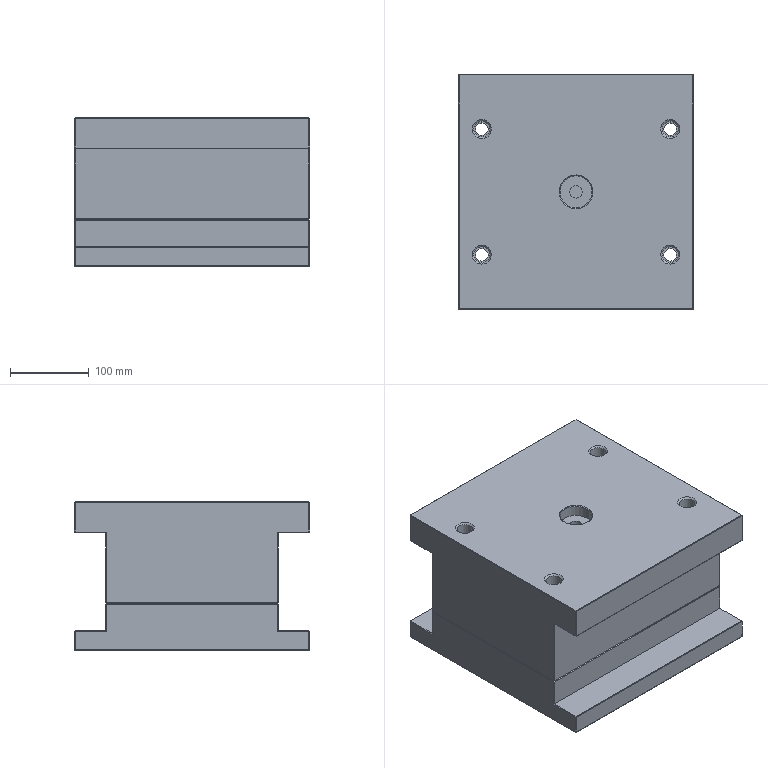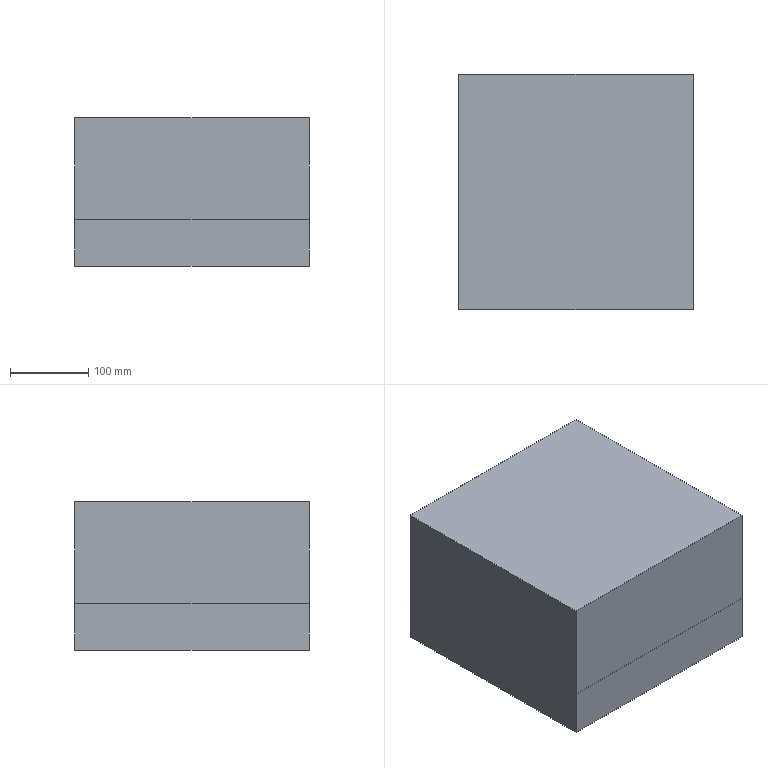CAM job | NX | 3-axis milling, drilling | part box 300 x 300 x 190 mm | stock box 300 x 300 x 190 mm
Tools:
number,name,description,diameter,corner_radius,flute_length,length,flutes
7,D6A45,Milling Tool-5 Parameters,6.0,0.0,50.0,75.0,2
1,ZXZ,Milling Tool-5 Parameters,6.0,0.0,50.0,75.0,2
11,10.ZT,Drilling Tool,10.0,0.0,35.0,50.0,2
2,D25R5,Milling Tool-5 Parameters,25.0,5.0,50.0,75.0,2
10,D10C,Milling Tool-5 Parameters,10.0,0.0,50.0,75.0,2
9,D10JING,Milling Tool-5 Parameters,10.0,0.0,50.0,75.0,2
12,R3,Milling Tool-5 Parameters,6.0,3.0,50.0,75.0,2
6,D6,Milling Tool-5 Parameters,6.0,0.0,50.0,75.0,2
15,D25R0.8,Milling Tool-5 Parameters,25.0,0.8,50.0,75.0,2
Operations:
program,operation,operation_type,tool,method,geometry_group,spindle_rpm,surface_speed,feed_per_tooth,feed_cut,feed_plunge,cut_length_mm,path_length_mm,cut_time_min,machine_time_min
1,DRILLING,Operation,ZXZ,METHOD,A,3500.0,65.0,0.0286,200.0,0.0,20.0,720.563,0.1,0.1701
1,DRILLING_1,Operation,10.ZT,METHOD,A,1200.0,37.0,0.05,120.0,0.0,268.017,1165.109,2.233,2.323
1,CAVITY_MILL,CavityMilling,D25R5,METHOD,A,1000.0,78.0,1.0,2000.0,1000.0,41589.871,44517.635,22.589,22.882
1,FLOOR_WALL,VolumeBased25DMillingOperation,D25R5,METHOD,A,1000.0,0.0,0.0,2000.0,1000.0,248046.214,253706.579,125.799,126.365
1,CAVITY_MILL_COPY,CavityMilling,D10C,METHOD,A,2500.0,78.0,0.4,2000.0,1000.0,24468.781,47953.241,12.498,14.847
1,HOLE_MILLING,CylinderMilling,D10C,METHOD,A,2000.0,62.0,0.375,1500.0,100.0,22158.353,23196.353,14.772,14.876
1,FLOOR_WALL_1,VolumeBased25DMillingOperation,D10JING,METHOD,A,4000.0,125.0,0.15,1200.0,100.0,5645.915,6426.663,4.705,4.783
1,FLOOR_WALL_1_COPY,VolumeBased25DMillingOperation,D10JING,METHOD,A,4000.0,125.0,0.15,1200.0,100.0,3960.323,4457.6,3.3,3.35
1,PLANAR_MILL,PlanarMilling,D6A45,METHOD,A,7500.0,141.0,0.0833,1250.0,100.0,1255.392,2137.648,1.004,1.093
1,PLANAR_MILL_COPY,PlanarMilling,D6A45,METHOD,A,7500.0,141.0,0.0833,1250.0,100.0,732.197,1579.963,0.5858,0.6705
1,刀补,CylinderMilling,D10JING,METHOD,A,3500.0,109.0,0.1714,1200.0,100.0,1921.866,2959.866,1.602,1.705
1,刀补2,VolumeBased25DMillingOperation,D10JING,METHOD,A,4000.0,125.0,0.15,1200.0,100.0,555.058,922.713,0.4625,0.4993
2,HOLE_MILLING_COPY,CylinderMilling,D10C,METHOD,B,2000.0,62.0,0.375,1500.0,100.0,8256.328,9188.328,5.504,5.597
2,PLANAR_MILL_COPY_1,PlanarMilling,D6A45,METHOD,B,7500.0,141.0,0.0833,1250.0,100.0,284.271,1084.278,0.2274,0.3074
3-1,DRILLING_COPY,Operation,ZXZ,METHOD,C,3500.0,65.0,0.0286,200.0,0.0,20.0,720.563,0.1,0.1701
3-2,DRILLING_1_COPY,Operation,10.ZT,METHOD,C,1200.0,37.0,0.05,120.0,0.0,268.017,1165.109,2.233,2.323
3-3,CAVITY_MILL_COPY_1,CavityMilling,D25R5,METHOD,C,1000.0,78.0,1.0,2000.0,1000.0,84406.834,90506.334,46.64,47.25
3-3,FLOOR_WALL_COPY,VolumeBased25DMillingOperation,D25R5,METHOD,C,1000.0,0.0,0.0,2000.0,1000.0,637478.771,651451.654,323.305,324.702
3-4,CAVITY_MILL_COPY_COPY_COPY,CavityMilling,D6,METHOD,C,2500.0,78.0,0.3,1500.0,1000.0,83354.416,90533.421,59.664,60.382
3-5,FLOOR_WALL_1_COPY_1_COPY,VolumeBased25DMillingOperation,D25R0.8,METHOD,C,4000.0,125.0,0.1,800.0,100.0,55226.401,135980.548,69.033,77.108
3-5,FLOOR_WALL_1_COPY_1,VolumeBased25DMillingOperation,D25R0.8,METHOD,C,4000.0,125.0,0.1,800.0,100.0,3326.228,4559.812,4.158,4.281
3-6,PLANAR_MILL_COPY_2,PlanarMilling,D6A45,METHOD,C,7500.0,141.0,0.0833,1250.0,100.0,1255.392,2141.632,1.004,1.093
3-6,PLANAR_MILL_COPY_COPY,PlanarMilling,D6A45,METHOD,C,7500.0,141.0,0.0833,1250.0,100.0,759.224,1468.107,0.6074,0.6783
3-7,HOLE_MILLING_COPY_1,CylinderMilling,D10C,METHOD,C,2000.0,62.0,0.2,800.0,100.0,22081.954,23119.954,27.602,27.706
3-8,ZLEVEL_PROFILE,ZLevelMilling,R3,METHOD,C,7500.0,235.0,0.1667,2500.0,100.0,173371.268,173782.694,69.349,69.39
3-9,刀补_COPY,CylinderMilling,D10JING,METHOD,C,3500.0,109.0,0.1714,1200.0,100.0,1930.374,2970.374,1.609,1.713
4-1,DRILLING_COPY_1,Operation,ZXZ,METHOD,D,3500.0,65.0,0.0286,200.0,0.0,20.0,720.563,0.1,0.1701
4-2,DRILLING_1_COPY_1,Operation,10.ZT,METHOD,D,1200.0,37.0,0.05,120.0,0.0,304.017,1237.109,2.534,2.627
4-2,DRILLING_1_COPY_1_COPY,Operation,10.ZT,METHOD,D,1200.0,37.0,0.05,120.0,0.0,29.0,118.0,0.2417,0.2506
4-3,HOLE_MILLING_COPY_2,CylinderMilling,D10C,METHOD,D,2000.0,62.0,0.2,800.0,100.0,44485.85,45563.85,55.607,55.715
4-3,HOLE_MILLING_COPY_3,CylinderMilling,D10C,METHOD,D,2000.0,62.0,0.375,1500.0,100.0,19110.442,19231.442,12.74,12.752
4-3,HOLE_MILLING_COPY_3_COPY,CylinderMilling,D10C,METHOD,D,2000.0,62.0,0.375,1500.0,100.0,1080.788,1181.35,0.7205,0.7306
4-4,PLANAR_MILL_COPY_3,PlanarMilling,D6A45,METHOD,D,7500.0,141.0,0.0833,1250.0,100.0,415.029,1322.143,0.332,0.4227
4-5,刀补_COPY_1,CylinderMilling,D10JING,METHOD,D,3500.0,109.0,0.1714,1200.0,100.0,734.519,809.019,0.6121,0.6195
4-5,刀补_COPY_1_COPY,CylinderMilling,D10JING,METHOD,D,3500.0,109.0,0.1714,1200.0,100.0,114.349,214.911,0.0953,0.1053